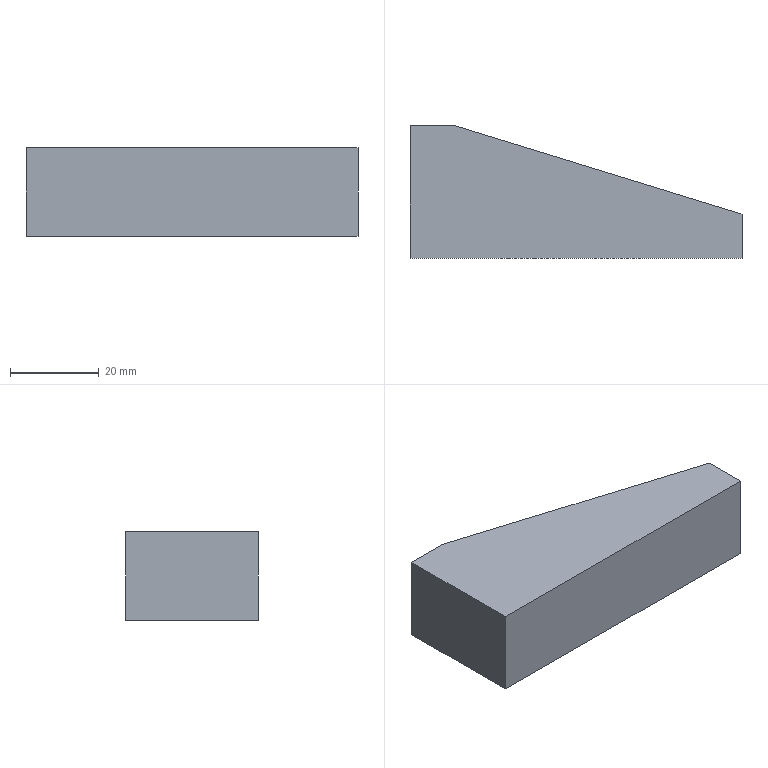Part | NX | 1 solid | 7 faces | box 75 x 30 x 20 mm | volume 32000 mm3 | plane 7
STEP:
#1=CARTESIAN_POINT('',(0.,0.,-10.));
#2=VERTEX_POINT('',#1);
#3=CARTESIAN_POINT('',(75.,0.,-10.));
#4=VERTEX_POINT('',#3);
#5=CARTESIAN_POINT('',(0.,0.,-10.));
#6=DIRECTION('',(1.,0.,0.));
#7=VECTOR('',#6,1000.);
#8=LINE('',#5,#7);
#9=EDGE_CURVE('',#2,#4,#8,.T.);
#10=ORIENTED_EDGE('',*,*,#9,.T.);
#11=CARTESIAN_POINT('',(75.,0.,10.));
#12=VERTEX_POINT('',#11);
#13=CARTESIAN_POINT('',(75.,0.,10.));
#14=DIRECTION('',(0.,0.,-1.));
#15=VECTOR('',#14,1000.);
#16=LINE('',#13,#15);
#17=EDGE_CURVE('',#12,#4,#16,.T.);
#18=ORIENTED_EDGE('',*,*,#17,.F.);
#19=CARTESIAN_POINT('',(0.,0.,10.));
#20=VERTEX_POINT('',#19);
#21=CARTESIAN_POINT('',(0.,0.,10.));
#22=DIRECTION('',(1.,0.,0.));
#23=VECTOR('',#22,1000.);
#24=LINE('',#21,#23);
#25=EDGE_CURVE('',#20,#12,#24,.T.);
#26=ORIENTED_EDGE('',*,*,#25,.F.);
#27=CARTESIAN_POINT('',(0.,0.,10.));
#28=DIRECTION('',(0.,0.,-1.));
#29=VECTOR('',#28,1000.);
#30=LINE('',#27,#29);
#31=EDGE_CURVE('',#20,#2,#30,.T.);
#32=ORIENTED_EDGE('',*,*,#31,.T.);
#33=EDGE_LOOP('',(#10,#18,#26,#32));
#34=FACE_BOUND('',#33,.T.);
#35=CARTESIAN_POINT('',(0.,0.,10.));
#36=DIRECTION('',(0.,1.,0.));
#37=DIRECTION('',(0.,0.,1.));
#38=AXIS2_PLACEMENT_3D('',#35,#36,#37);
#39=PLANE('',#38);
#40=ADVANCED_FACE('',(#34),#39,.F.);
#41=CARTESIAN_POINT('',(75.,10.,-10.));
#42=VERTEX_POINT('',#41);
#43=CARTESIAN_POINT('',(75.,0.,-10.));
#44=DIRECTION('',(0.,1.,0.));
#45=VECTOR('',#44,1000.);
#46=LINE('',#43,#45);
#47=EDGE_CURVE('',#4,#42,#46,.T.);
#48=ORIENTED_EDGE('',*,*,#47,.T.);
#49=CARTESIAN_POINT('',(75.,10.,10.));
#50=VERTEX_POINT('',#49);
#51=CARTESIAN_POINT('',(75.,10.,10.));
#52=DIRECTION('',(0.,0.,-1.));
#53=VECTOR('',#52,1000.);
#54=LINE('',#51,#53);
#55=EDGE_CURVE('',#50,#42,#54,.T.);
#56=ORIENTED_EDGE('',*,*,#55,.F.);
#57=CARTESIAN_POINT('',(75.,0.,10.));
#58=DIRECTION('',(0.,1.,0.));
#59=VECTOR('',#58,1000.);
#60=LINE('',#57,#59);
#61=EDGE_CURVE('',#12,#50,#60,.T.);
#62=ORIENTED_EDGE('',*,*,#61,.F.);
#63=ORIENTED_EDGE('',*,*,#17,.T.);
#64=EDGE_LOOP('',(#48,#56,#62,#63));
#65=FACE_BOUND('',#64,.T.);
#66=CARTESIAN_POINT('',(75.,0.,10.));
#67=DIRECTION('',(-1.,0.,0.));
#68=DIRECTION('',(0.,0.,1.));
#69=AXIS2_PLACEMENT_3D('',#66,#67,#68);
#70=PLANE('',#69);
#71=ADVANCED_FACE('',(#65),#70,.F.);
#72=CARTESIAN_POINT('',(10.,30.,-10.));
#73=VERTEX_POINT('',#72);
#74=CARTESIAN_POINT('',(10.,30.,-10.));
#75=DIRECTION('',(-0.9558,0.2941,0.));
#76=VECTOR('',#75,1000.);
#77=LINE('',#74,#76);
#78=EDGE_CURVE('',#42,#73,#77,.T.);
#79=ORIENTED_EDGE('',*,*,#78,.T.);
#80=CARTESIAN_POINT('',(10.,30.,10.));
#81=VERTEX_POINT('',#80);
#82=CARTESIAN_POINT('',(10.,30.,10.));
#83=DIRECTION('',(0.,0.,-1.));
#84=VECTOR('',#83,1000.);
#85=LINE('',#82,#84);
#86=EDGE_CURVE('',#81,#73,#85,.T.);
#87=ORIENTED_EDGE('',*,*,#86,.F.);
#88=CARTESIAN_POINT('',(10.,30.,10.));
#89=DIRECTION('',(-0.9558,0.2941,0.));
#90=VECTOR('',#89,1000.);
#91=LINE('',#88,#90);
#92=EDGE_CURVE('',#50,#81,#91,.T.);
#93=ORIENTED_EDGE('',*,*,#92,.F.);
#94=ORIENTED_EDGE('',*,*,#55,.T.);
#95=EDGE_LOOP('',(#79,#87,#93,#94));
#96=FACE_BOUND('',#95,.T.);
#97=CARTESIAN_POINT('',(10.,30.,10.));
#98=DIRECTION('',(-0.2941,-0.9558,0.));
#99=DIRECTION('',(0.9558,-0.2941,0.));
#100=AXIS2_PLACEMENT_3D('',#97,#98,#99);
#101=PLANE('',#100);
#102=ADVANCED_FACE('',(#96),#101,.F.);
#103=CARTESIAN_POINT('',(0.,30.,-10.));
#104=VERTEX_POINT('',#103);
#105=CARTESIAN_POINT('',(0.,30.,-10.));
#106=DIRECTION('',(-1.,0.,0.));
#107=VECTOR('',#106,1000.);
#108=LINE('',#105,#107);
#109=EDGE_CURVE('',#73,#104,#108,.T.);
#110=ORIENTED_EDGE('',*,*,#109,.T.);
#111=CARTESIAN_POINT('',(0.,30.,10.));
#112=VERTEX_POINT('',#111);
#113=CARTESIAN_POINT('',(0.,30.,10.));
#114=DIRECTION('',(0.,0.,-1.));
#115=VECTOR('',#114,1000.);
#116=LINE('',#113,#115);
#117=EDGE_CURVE('',#112,#104,#116,.T.);
#118=ORIENTED_EDGE('',*,*,#117,.F.);
#119=CARTESIAN_POINT('',(0.,30.,10.));
#120=DIRECTION('',(-1.,0.,0.));
#121=VECTOR('',#120,1000.);
#122=LINE('',#119,#121);
#123=EDGE_CURVE('',#81,#112,#122,.T.);
#124=ORIENTED_EDGE('',*,*,#123,.F.);
#125=ORIENTED_EDGE('',*,*,#86,.T.);
#126=EDGE_LOOP('',(#110,#118,#124,#125));
#127=FACE_BOUND('',#126,.T.);
#128=CARTESIAN_POINT('',(0.,30.,10.));
#129=DIRECTION('',(0.,-1.,0.));
#130=DIRECTION('',(0.,0.,-1.));
#131=AXIS2_PLACEMENT_3D('',#128,#129,#130);
#132=PLANE('',#131);
#133=ADVANCED_FACE('',(#127),#132,.F.);
#134=CARTESIAN_POINT('',(0.,0.,-10.));
#135=DIRECTION('',(0.,-1.,0.));
#136=VECTOR('',#135,1000.);
#137=LINE('',#134,#136);
#138=EDGE_CURVE('',#104,#2,#137,.T.);
#139=ORIENTED_EDGE('',*,*,#138,.T.);
#140=ORIENTED_EDGE('',*,*,#31,.F.);
#141=CARTESIAN_POINT('',(0.,0.,10.));
#142=DIRECTION('',(0.,-1.,0.));
#143=VECTOR('',#142,1000.);
#144=LINE('',#141,#143);
#145=EDGE_CURVE('',#112,#20,#144,.T.);
#146=ORIENTED_EDGE('',*,*,#145,.F.);
#147=ORIENTED_EDGE('',*,*,#117,.T.);
#148=EDGE_LOOP('',(#139,#140,#146,#147));
#149=FACE_BOUND('',#148,.T.);
#150=CARTESIAN_POINT('',(0.,0.,10.));
#151=DIRECTION('',(1.,0.,0.));
#152=DIRECTION('',(0.,0.,-1.));
#153=AXIS2_PLACEMENT_3D('',#150,#151,#152);
#154=PLANE('',#153);
#155=ADVANCED_FACE('',(#149),#154,.F.);
#156=ORIENTED_EDGE('',*,*,#25,.T.);
#157=ORIENTED_EDGE('',*,*,#61,.T.);
#158=ORIENTED_EDGE('',*,*,#92,.T.);
#159=ORIENTED_EDGE('',*,*,#123,.T.);
#160=ORIENTED_EDGE('',*,*,#145,.T.);
#161=EDGE_LOOP('',(#156,#157,#158,#159,#160));
#162=FACE_BOUND('',#161,.T.);
#163=CARTESIAN_POINT('',(0.,0.,10.));
#164=DIRECTION('',(0.,0.,1.));
#165=DIRECTION('',(1.,0.,0.));
#166=AXIS2_PLACEMENT_3D('',#163,#164,#165);
#167=PLANE('',#166);
#168=ADVANCED_FACE('',(#162),#167,.T.);
#169=ORIENTED_EDGE('',*,*,#9,.F.);
#170=ORIENTED_EDGE('',*,*,#138,.F.);
#171=ORIENTED_EDGE('',*,*,#109,.F.);
#172=ORIENTED_EDGE('',*,*,#78,.F.);
#173=ORIENTED_EDGE('',*,*,#47,.F.);
#174=EDGE_LOOP('',(#169,#170,#171,#172,#173));
#175=FACE_BOUND('',#174,.T.);
#176=CARTESIAN_POINT('',(0.,0.,-10.));
#177=DIRECTION('',(0.,0.,1.));
#178=DIRECTION('',(1.,0.,0.));
#179=AXIS2_PLACEMENT_3D('',#176,#177,#178);
#180=PLANE('',#179);
#181=ADVANCED_FACE('',(#175),#180,.F.);
#182=CLOSED_SHELL('',(#40,#71,#102,#133,#155,#168,#181));
#183=MANIFOLD_SOLID_BREP('',#182);
#184=(LENGTH_UNIT()NAMED_UNIT(*)SI_UNIT(.MILLI.,.METRE.));
#185=UNCERTAINTY_MEASURE_WITH_UNIT(LENGTH_MEASURE(0.00001),#184,'','');
#186=(NAMED_UNIT(*)PLANE_ANGLE_UNIT()SI_UNIT($,.RADIAN.));
#187=(NAMED_UNIT(*)SI_UNIT($,.STERADIAN.)SOLID_ANGLE_UNIT());
#188=(GEOMETRIC_REPRESENTATION_CONTEXT(3)GLOBAL_UNCERTAINTY_ASSIGNED_CONTEXT((#185))GLOBAL_UNIT_ASSIGNED_CONTEXT((#184,#186,#187))REPRESENTATION_CONTEXT('',''));
#189=ADVANCED_BREP_SHAPE_REPRESENTATION('',(#183),#188);